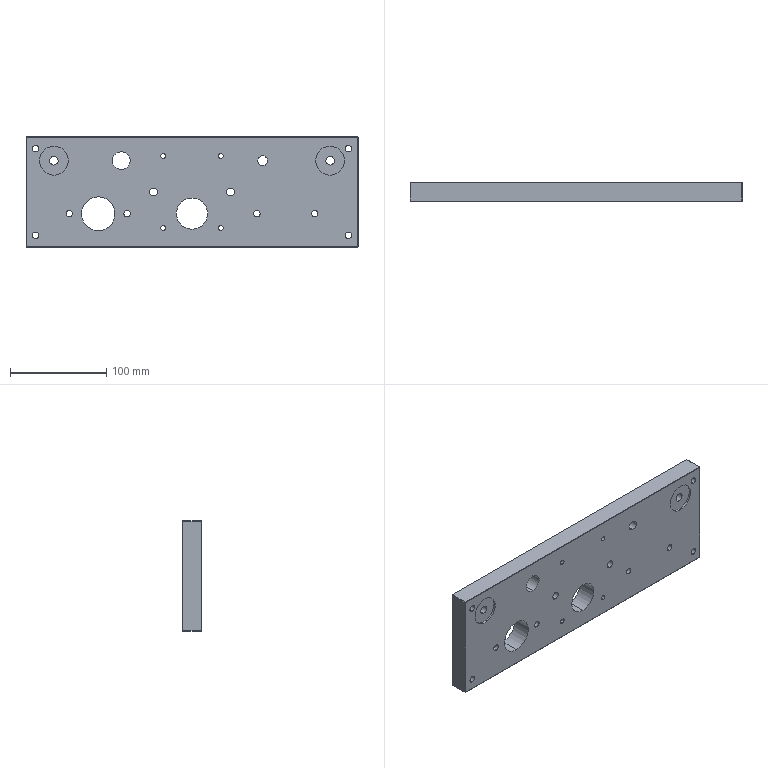Part | STEP file | 11-FG-SJ00111 | 1 solid | 90 faces | box 345 x 20 x 115 mm | volume 732573 mm3 | cylinder 56 | plane 34 | commonest cylinder face diameters 5 x8 6.6 x8 6.8 x8 11 x8 8 x4 9 x4